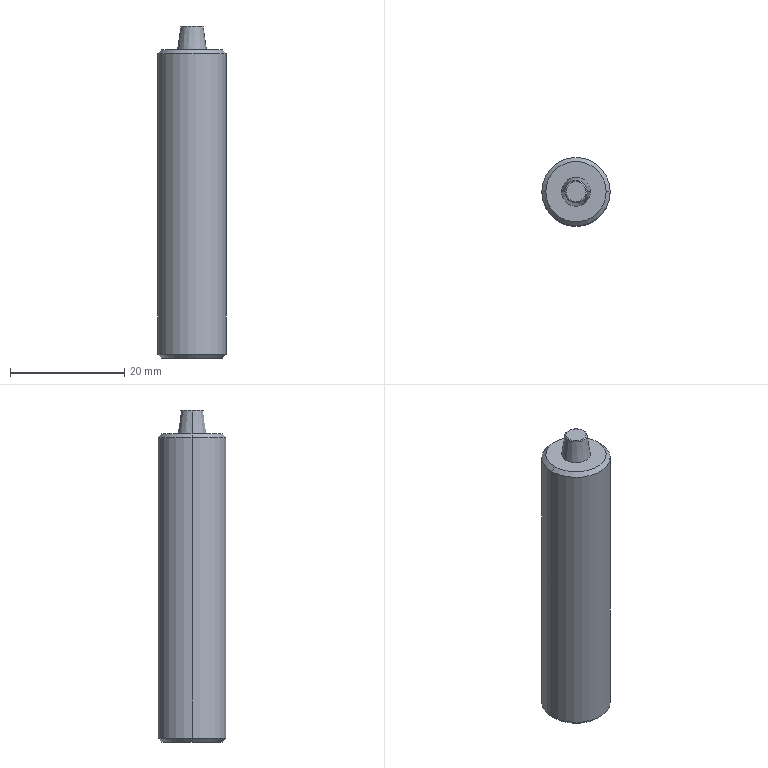Part | SolidWorks | features RefAxis 21, 3DProfileFeature 7, Revolution 3, ICE 2, RevCut 2 | 1 solid | 39 faces | box 12 x 12 x 58.2 mm | volume 5676 mm3 | plane 23 | cone 10 | cylinder 4 | torus 2 | commonest cylinder face diameters 6.917 x2 12 x2
STEP:
#1=CARTESIAN_POINT('',(0.,0.,-40.845));
#2=VERTEX_POINT('',#1);
#3=CARTESIAN_POINT('',(-2.,0.,-42.));
#4=VERTEX_POINT('',#3);
#5=CARTESIAN_POINT('',(-2.,0.,-42.));
#6=DIRECTION('',(-0.866,0.,-0.5));
#7=VECTOR('',#6,1000.);
#8=LINE('',#5,#7);
#9=EDGE_CURVE('',#2,#4,#8,.T.);
#10=ORIENTED_EDGE('',*,*,#9,.F.);
#11=CARTESIAN_POINT('',(2.,0.,-42.));
#12=VERTEX_POINT('',#11);
#13=CARTESIAN_POINT('',(2.,0.,-42.));
#14=DIRECTION('',(0.866,0.,-0.5));
#15=VECTOR('',#14,1000.);
#16=LINE('',#13,#15);
#17=EDGE_CURVE('',#2,#12,#16,.T.);
#18=ORIENTED_EDGE('',*,*,#17,.T.);
#19=CARTESIAN_POINT('',(1.,-1.732,-42.));
#20=VERTEX_POINT('',#19);
#21=CARTESIAN_POINT('',(0.,0.,-42.));
#22=DIRECTION('',(0.,0.,-1.));
#23=DIRECTION('',(1.,0.,0.));
#24=AXIS2_PLACEMENT_3D('',#21,#22,#23);
#25=CIRCLE('',#24,2.);
#26=EDGE_CURVE('',#12,#20,#25,.T.);
#27=ORIENTED_EDGE('',*,*,#26,.T.);
#28=CARTESIAN_POINT('',(-1.,-1.732,-42.));
#29=VERTEX_POINT('',#28);
#30=CARTESIAN_POINT('',(0.,0.,-42.));
#31=DIRECTION('',(0.,0.,-1.));
#32=DIRECTION('',(1.,0.,0.));
#33=AXIS2_PLACEMENT_3D('',#30,#31,#32);
#34=CIRCLE('',#33,2.);
#35=EDGE_CURVE('',#20,#29,#34,.T.);
#36=ORIENTED_EDGE('',*,*,#35,.T.);
#37=CARTESIAN_POINT('',(0.,0.,-42.));
#38=DIRECTION('',(0.,0.,-1.));
#39=DIRECTION('',(1.,0.,0.));
#40=AXIS2_PLACEMENT_3D('',#37,#38,#39);
#41=CIRCLE('',#40,2.);
#42=EDGE_CURVE('',#29,#4,#41,.T.);
#43=ORIENTED_EDGE('',*,*,#42,.T.);
#44=EDGE_LOOP('',(#10,#18,#27,#36,#43));
#45=FACE_OUTER_BOUND('',#44,.T.);
#46=CARTESIAN_POINT('',(0.,0.,-42.));
#47=DIRECTION('',(0.,0.,-1.));
#48=DIRECTION('',(-1.,0.,0.));
#49=AXIS2_PLACEMENT_3D('',#46,#47,#48);
#50=CONICAL_SURFACE('',#49,2.,1.047);
#51=ADVANCED_FACE('',(#45),#50,.F.);
#52=CARTESIAN_POINT('',(1.961,0.,4.028));
#53=VERTEX_POINT('',#52);
#54=CARTESIAN_POINT('',(-1.961,0.,4.028));
#55=VERTEX_POINT('',#54);
#56=CARTESIAN_POINT('',(0.,0.,4.028));
#57=DIRECTION('',(0.,0.,1.));
#58=DIRECTION('',(1.,0.,0.));
#59=AXIS2_PLACEMENT_3D('',#56,#57,#58);
#60=CIRCLE('',#59,1.961);
#61=EDGE_CURVE('',#53,#55,#60,.T.);
#62=ORIENTED_EDGE('',*,*,#61,.T.);
#63=CARTESIAN_POINT('',(-1.763,0.,4.2));
#64=VERTEX_POINT('',#63);
#65=CARTESIAN_POINT('',(-1.763,0.,4.));
#66=DIRECTION('',(0.,1.,0.));
#67=DIRECTION('',(-1.,0.,0.));
#68=AXIS2_PLACEMENT_3D('',#65,#66,#67);
#69=CIRCLE('',#68,0.2);
#70=EDGE_CURVE('',#55,#64,#69,.T.);
#71=ORIENTED_EDGE('',*,*,#70,.T.);
#72=CARTESIAN_POINT('',(1.763,0.,4.2));
#73=VERTEX_POINT('',#72);
#74=CARTESIAN_POINT('',(0.,0.,4.2));
#75=DIRECTION('',(0.,0.,1.));
#76=DIRECTION('',(1.,0.,0.));
#77=AXIS2_PLACEMENT_3D('',#74,#75,#76);
#78=CIRCLE('',#77,1.763);
#79=EDGE_CURVE('',#73,#64,#78,.T.);
#80=ORIENTED_EDGE('',*,*,#79,.F.);
#81=CARTESIAN_POINT('',(1.763,0.,4.));
#82=DIRECTION('',(0.,-1.,0.));
#83=DIRECTION('',(0.,0.,-1.));
#84=AXIS2_PLACEMENT_3D('',#81,#82,#83);
#85=CIRCLE('',#84,0.2);
#86=EDGE_CURVE('',#53,#73,#85,.T.);
#87=ORIENTED_EDGE('',*,*,#86,.F.);
#88=EDGE_LOOP('',(#62,#71,#80,#87));
#89=FACE_OUTER_BOUND('',#88,.T.);
#90=CARTESIAN_POINT('',(0.,0.,4.));
#91=DIRECTION('',(0.,0.,1.));
#92=DIRECTION('',(1.,0.,0.));
#93=AXIS2_PLACEMENT_3D('',#90,#91,#92);
#94=TOROIDAL_SURFACE('',#93,1.763,0.2);
#95=ADVANCED_FACE('',(#89),#94,.T.);
#96=ORIENTED_EDGE('',*,*,#61,.F.);
#97=CARTESIAN_POINT('',(2.527,0.,0.));
#98=VERTEX_POINT('',#97);
#99=CARTESIAN_POINT('',(2.85,0.,-2.3));
#100=DIRECTION('',(0.1392,0.,-0.9903));
#101=VECTOR('',#100,1000.);
#102=LINE('',#99,#101);
#103=EDGE_CURVE('',#53,#98,#102,.T.);
#104=ORIENTED_EDGE('',*,*,#103,.T.);
#105=CARTESIAN_POINT('',(-2.527,0.,0.));
#106=VERTEX_POINT('',#105);
#107=CARTESIAN_POINT('',(0.,0.,0.));
#108=DIRECTION('',(0.,0.,1.));
#109=DIRECTION('',(-1.,0.,0.));
#110=AXIS2_PLACEMENT_3D('',#107,#108,#109);
#111=CIRCLE('',#110,2.527);
#112=EDGE_CURVE('',#98,#106,#111,.T.);
#113=ORIENTED_EDGE('',*,*,#112,.T.);
#114=CARTESIAN_POINT('',(-2.85,0.,-2.3));
#115=DIRECTION('',(-0.1392,0.,-0.9903));
#116=VECTOR('',#115,1000.);
#117=LINE('',#114,#116);
#118=EDGE_CURVE('',#55,#106,#117,.T.);
#119=ORIENTED_EDGE('',*,*,#118,.F.);
#120=EDGE_LOOP('',(#96,#104,#113,#119));
#121=FACE_OUTER_BOUND('',#120,.T.);
#122=CARTESIAN_POINT('',(0.,0.,-2.3));
#123=DIRECTION('',(0.,0.,-1.));
#124=DIRECTION('',(-1.,0.,0.));
#125=AXIS2_PLACEMENT_3D('',#122,#123,#124);
#126=CONICAL_SURFACE('',#125,2.85,0.1396);
#127=ADVANCED_FACE('',(#121),#126,.T.);
#128=CARTESIAN_POINT('',(5.3,0.,-54.));
#129=VERTEX_POINT('',#128);
#130=CARTESIAN_POINT('',(-5.3,0.,-54.));
#131=VERTEX_POINT('',#130);
#132=CARTESIAN_POINT('',(0.,0.,-54.));
#133=DIRECTION('',(0.,0.,1.));
#134=DIRECTION('',(1.,0.,0.));
#135=AXIS2_PLACEMENT_3D('',#132,#133,#134);
#136=CIRCLE('',#135,5.3);
#137=EDGE_CURVE('',#129,#131,#136,.T.);
#138=ORIENTED_EDGE('',*,*,#137,.T.);
#139=CARTESIAN_POINT('',(-6.,0.,-53.3));
#140=VERTEX_POINT('',#139);
#141=CARTESIAN_POINT('',(-5.3,0.,-54.));
#142=DIRECTION('',(-0.7071,0.,0.7071));
#143=VECTOR('',#142,1000.);
#144=LINE('',#141,#143);
#145=EDGE_CURVE('',#131,#140,#144,.T.);
#146=ORIENTED_EDGE('',*,*,#145,.T.);
#147=CARTESIAN_POINT('',(6.,0.,-53.3));
#148=VERTEX_POINT('',#147);
#149=CARTESIAN_POINT('',(0.,0.,-53.3));
#150=DIRECTION('',(0.,0.,1.));
#151=DIRECTION('',(1.,0.,0.));
#152=AXIS2_PLACEMENT_3D('',#149,#150,#151);
#153=CIRCLE('',#152,6.);
#154=EDGE_CURVE('',#148,#140,#153,.T.);
#155=ORIENTED_EDGE('',*,*,#154,.F.);
#156=CARTESIAN_POINT('',(5.3,0.,-54.));
#157=DIRECTION('',(0.7071,0.,0.7071));
#158=VECTOR('',#157,1000.);
#159=LINE('',#156,#158);
#160=EDGE_CURVE('',#129,#148,#159,.T.);
#161=ORIENTED_EDGE('',*,*,#160,.F.);
#162=EDGE_LOOP('',(#138,#146,#155,#161));
#163=FACE_OUTER_BOUND('',#162,.T.);
#164=CARTESIAN_POINT('',(0.,0.,-54.));
#165=DIRECTION('',(0.,0.,1.));
#166=DIRECTION('',(1.,0.,0.));
#167=AXIS2_PLACEMENT_3D('',#164,#165,#166);
#168=CONICAL_SURFACE('',#167,5.3,0.7854);
#169=ADVANCED_FACE('',(#163),#168,.T.);
#170=ORIENTED_EDGE('',*,*,#154,.T.);
#171=CARTESIAN_POINT('',(-6.,0.,-0.7));
#172=VERTEX_POINT('',#171);
#173=CARTESIAN_POINT('',(-6.,0.,-54.));
#174=DIRECTION('',(0.,0.,1.));
#175=VECTOR('',#174,1000.);
#176=LINE('',#173,#175);
#177=EDGE_CURVE('',#140,#172,#176,.T.);
#178=ORIENTED_EDGE('',*,*,#177,.T.);
#179=CARTESIAN_POINT('',(6.,0.,-0.7));
#180=VERTEX_POINT('',#179);
#181=CARTESIAN_POINT('',(0.,0.,-0.7));
#182=DIRECTION('',(0.,0.,1.));
#183=DIRECTION('',(1.,0.,0.));
#184=AXIS2_PLACEMENT_3D('',#181,#182,#183);
#185=CIRCLE('',#184,6.);
#186=EDGE_CURVE('',#180,#172,#185,.T.);
#187=ORIENTED_EDGE('',*,*,#186,.F.);
#188=CARTESIAN_POINT('',(6.,0.,-54.));
#189=DIRECTION('',(0.,0.,1.));
#190=VECTOR('',#189,1000.);
#191=LINE('',#188,#190);
#192=EDGE_CURVE('',#148,#180,#191,.T.);
#193=ORIENTED_EDGE('',*,*,#192,.F.);
#194=EDGE_LOOP('',(#170,#178,#187,#193));
#195=FACE_OUTER_BOUND('',#194,.T.);
#196=CARTESIAN_POINT('',(0.,0.,-54.));
#197=DIRECTION('',(0.,0.,1.));
#198=DIRECTION('',(1.,0.,0.));
#199=AXIS2_PLACEMENT_3D('',#196,#197,#198);
#200=CYLINDRICAL_SURFACE('',#199,6.);
#201=ADVANCED_FACE('',(#195),#200,.T.);
#202=CARTESIAN_POINT('',(5.3,0.,0.));
#203=VERTEX_POINT('',#202);
#204=CARTESIAN_POINT('',(-5.3,0.,0.));
#205=VERTEX_POINT('',#204);
#206=CARTESIAN_POINT('',(0.,0.,0.));
#207=DIRECTION('',(0.,0.,1.));
#208=DIRECTION('',(1.,0.,0.));
#209=AXIS2_PLACEMENT_3D('',#206,#207,#208);
#210=CIRCLE('',#209,5.3);
#211=EDGE_CURVE('',#203,#205,#210,.T.);
#212=ORIENTED_EDGE('',*,*,#211,.F.);
#213=CARTESIAN_POINT('',(6.,0.,-0.7));
#214=DIRECTION('',(0.7071,0.,-0.7071));
#215=VECTOR('',#214,1000.);
#216=LINE('',#213,#215);
#217=EDGE_CURVE('',#203,#180,#216,.T.);
#218=ORIENTED_EDGE('',*,*,#217,.T.);
#219=ORIENTED_EDGE('',*,*,#186,.T.);
#220=CARTESIAN_POINT('',(-6.,0.,-0.7));
#221=DIRECTION('',(-0.7071,0.,-0.7071));
#222=VECTOR('',#221,1000.);
#223=LINE('',#220,#222);
#224=EDGE_CURVE('',#205,#172,#223,.T.);
#225=ORIENTED_EDGE('',*,*,#224,.F.);
#226=EDGE_LOOP('',(#212,#218,#219,#225));
#227=FACE_OUTER_BOUND('',#226,.T.);
#228=CARTESIAN_POINT('',(0.,0.,-0.7));
#229=DIRECTION('',(0.,0.,-1.));
#230=DIRECTION('',(-1.,0.,0.));
#231=AXIS2_PLACEMENT_3D('',#228,#229,#230);
#232=CONICAL_SURFACE('',#231,6.,0.7854);
#233=ADVANCED_FACE('',(#227),#232,.T.);
#234=CARTESIAN_POINT('',(4.,-2.309,-53.819));
#235=VERTEX_POINT('',#234);
#236=CARTESIAN_POINT('',(4.,0.,-53.2));
#237=VERTEX_POINT('',#236);
#238=CARTESIAN_POINT('',(4.,-2.309,-53.819));
#239=CARTESIAN_POINT('',(4.,-1.951,-53.64));
#240=CARTESIAN_POINT('',(4.,-1.574,-53.483));
#241=CARTESIAN_POINT('',(4.,-0.9966,-53.318));
#242=CARTESIAN_POINT('',(4.,-0.8015,-53.275));
#243=CARTESIAN_POINT('',(4.,-0.4053,-53.216));
#244=CARTESIAN_POINT('',(4.,-0.2027,-53.2));
#245=CARTESIAN_POINT('',(4.,0.,-53.2));
#246=B_SPLINE_CURVE_WITH_KNOTS('',3,(#238,#239,#240,#241,#242,#243,#244,#245),.UNSPECIFIED.,.F.,.F.,(4,2,2,4),(0.003092,0.004289,0.004887,0.005485),.UNSPECIFIED.);
#247=EDGE_CURVE('',#235,#237,#246,.T.);
#248=ORIENTED_EDGE('',*,*,#247,.T.);
#249=CARTESIAN_POINT('',(4.8,0.,-54.));
#250=VERTEX_POINT('',#249);
#251=CARTESIAN_POINT('',(4.8,0.,-54.));
#252=DIRECTION('',(0.7071,0.,-0.7071));
#253=VECTOR('',#252,1000.);
#254=LINE('',#251,#253);
#255=EDGE_CURVE('',#237,#250,#254,.T.);
#256=ORIENTED_EDGE('',*,*,#255,.T.);
#257=CARTESIAN_POINT('',(-4.8,0.,-54.));
#258=VERTEX_POINT('',#257);
#259=CARTESIAN_POINT('',(0.,0.,-54.));
#260=DIRECTION('',(0.,0.,1.));
#261=DIRECTION('',(1.,0.,0.));
#262=AXIS2_PLACEMENT_3D('',#259,#260,#261);
#263=CIRCLE('',#262,4.8);
#264=EDGE_CURVE('',#258,#250,#263,.T.);
#265=ORIENTED_EDGE('',*,*,#264,.F.);
#266=CARTESIAN_POINT('',(-4.,0.,-53.2));
#267=VERTEX_POINT('',#266);
#268=CARTESIAN_POINT('',(-4.8,0.,-54.));
#269=DIRECTION('',(-0.7071,0.,-0.7071));
#270=VECTOR('',#269,1000.);
#271=LINE('',#268,#270);
#272=EDGE_CURVE('',#267,#258,#271,.T.);
#273=ORIENTED_EDGE('',*,*,#272,.F.);
#274=CARTESIAN_POINT('',(-4.,-2.309,-53.819));
#275=VERTEX_POINT('',#274);
#276=CARTESIAN_POINT('',(-4.,0.,-53.2));
#277=CARTESIAN_POINT('',(-4.,-0.2027,-53.2));
#278=CARTESIAN_POINT('',(-4.,-0.4053,-53.216));
#279=CARTESIAN_POINT('',(-4.,-0.8015,-53.275));
#280=CARTESIAN_POINT('',(-4.,-0.9966,-53.318));
#281=CARTESIAN_POINT('',(-4.,-1.574,-53.483));
#282=CARTESIAN_POINT('',(-4.,-1.951,-53.64));
#283=CARTESIAN_POINT('',(-4.,-2.309,-53.819));
#284=B_SPLINE_CURVE_WITH_KNOTS('',3,(#276,#277,#278,#279,#280,#281,#282,#283),.UNSPECIFIED.,.F.,.F.,(4,2,2,4),(0.004837,0.005435,0.006033,0.007228),.UNSPECIFIED.);
#285=EDGE_CURVE('',#267,#275,#284,.T.);
#286=ORIENTED_EDGE('',*,*,#285,.T.);
#287=CARTESIAN_POINT('',(0.,-4.619,-53.819));
#288=VERTEX_POINT('',#287);
#289=CARTESIAN_POINT('',(-4.,-2.309,-53.819));
#290=CARTESIAN_POINT('',(-3.687,-2.49,-53.638));
#291=CARTESIAN_POINT('',(-3.368,-2.674,-53.485));
#292=CARTESIAN_POINT('',(-2.871,-2.961,-53.321));
#293=CARTESIAN_POINT('',(-2.703,-3.058,-53.277));
#294=CARTESIAN_POINT('',(-2.359,-3.257,-53.217));
#295=CARTESIAN_POINT('',(-2.182,-3.359,-53.2));
#296=CARTESIAN_POINT('',(-1.658,-3.661,-53.199));
#297=CARTESIAN_POINT('',(-1.315,-3.86,-53.26));
#298=CARTESIAN_POINT('',(-0.6381,-4.25,-53.482));
#299=CARTESIAN_POINT('',(-0.3144,-4.437,-53.637));
#300=CARTESIAN_POINT('',(0.,-4.619,-53.819));
#301=B_SPLINE_CURVE_WITH_KNOTS('',3,(#289,#290,#291,#292,#293,#294,#295,#296,#297,#298,#299,#300),.UNSPECIFIED.,.F.,.F.,(4,2,2,2,2,4),(0.000000254,0.001193,0.001789,0.002386,0.003579,0.004771),.UNSPECIFIED.);
#302=EDGE_CURVE('',#275,#288,#301,.T.);
#303=ORIENTED_EDGE('',*,*,#302,.T.);
#304=CARTESIAN_POINT('',(0.,-4.619,-53.819));
#305=CARTESIAN_POINT('',(0.3125,-4.438,-53.638));
#306=CARTESIAN_POINT('',(0.6321,-4.254,-53.485));
#307=CARTESIAN_POINT('',(1.129,-3.967,-53.321));
#308=CARTESIAN_POINT('',(1.297,-3.87,-53.277));
#309=CARTESIAN_POINT('',(1.641,-3.671,-53.217));
#310=CARTESIAN_POINT('',(1.818,-3.569,-53.2));
#311=CARTESIAN_POINT('',(2.342,-3.267,-53.199));
#312=CARTESIAN_POINT('',(2.685,-3.069,-53.26));
#313=CARTESIAN_POINT('',(3.362,-2.678,-53.482));
#314=CARTESIAN_POINT('',(3.686,-2.491,-53.637));
#315=CARTESIAN_POINT('',(4.,-2.309,-53.819));
#316=B_SPLINE_CURVE_WITH_KNOTS('',3,(#304,#305,#306,#307,#308,#309,#310,#311,#312,#313,#314,#315),.UNSPECIFIED.,.F.,.F.,(4,2,2,2,2,4),(0.000000254,0.001193,0.001789,0.002386,0.003579,0.004771),.UNSPECIFIED.);
#317=EDGE_CURVE('',#288,#235,#316,.T.);
#318=ORIENTED_EDGE('',*,*,#317,.T.);
#319=EDGE_LOOP('',(#248,#256,#265,#273,#286,#303,#318));
#320=FACE_OUTER_BOUND('',#319,.T.);
#321=CARTESIAN_POINT('',(0.,0.,-54.));
#322=DIRECTION('',(0.,0.,-1.));
#323=DIRECTION('',(-1.,0.,0.));
#324=AXIS2_PLACEMENT_3D('',#321,#322,#323);
#325=CONICAL_SURFACE('',#324,4.8,0.7854);
#326=ADVANCED_FACE('',(#320),#325,.F.);
#327=CARTESIAN_POINT('',(-3.458,0.,-49.));
#328=VERTEX_POINT('',#327);
#329=CARTESIAN_POINT('',(3.458,0.,-49.));
#330=VERTEX_POINT('',#329);
#331=CARTESIAN_POINT('',(0.,0.,-49.));
#332=DIRECTION('',(0.,0.,1.));
#333=DIRECTION('',(1.,0.,0.));
#334=AXIS2_PLACEMENT_3D('',#331,#332,#333);
#335=CIRCLE('',#334,3.458);
#336=EDGE_CURVE('',#328,#330,#335,.T.);
#337=ORIENTED_EDGE('',*,*,#336,.F.);
#338=CARTESIAN_POINT('',(-3.458,0.,-45.));
#339=VERTEX_POINT('',#338);
#340=CARTESIAN_POINT('',(-3.458,0.,-54.));
#341=DIRECTION('',(0.,0.,1.));
#342=VECTOR('',#341,1000.);
#343=LINE('',#340,#342);
#344=EDGE_CURVE('',#328,#339,#343,.T.);
#345=ORIENTED_EDGE('',*,*,#344,.T.);
#346=CARTESIAN_POINT('',(3.458,0.,-45.));
#347=VERTEX_POINT('',#346);
#348=CARTESIAN_POINT('',(0.,0.,-45.));
#349=DIRECTION('',(0.,0.,1.));
#350=DIRECTION('',(1.,0.,0.));
#351=AXIS2_PLACEMENT_3D('',#348,#349,#350);
#352=CIRCLE('',#351,3.458);
#353=EDGE_CURVE('',#339,#347,#352,.T.);
#354=ORIENTED_EDGE('',*,*,#353,.T.);
#355=CARTESIAN_POINT('',(3.458,0.,-54.));
#356=DIRECTION('',(0.,0.,1.));
#357=VECTOR('',#356,1000.);
#358=LINE('',#355,#357);
#359=EDGE_CURVE('',#330,#347,#358,.T.);
#360=ORIENTED_EDGE('',*,*,#359,.F.);
#361=EDGE_LOOP('',(#337,#345,#354,#360));
#362=FACE_OUTER_BOUND('',#361,.T.);
#363=CARTESIAN_POINT('',(0.,0.,-54.));
#364=DIRECTION('',(0.,0.,1.));
#365=DIRECTION('',(1.,0.,0.));
#366=AXIS2_PLACEMENT_3D('',#363,#364,#365);
#367=CYLINDRICAL_SURFACE('',#366,3.458);
#368=ADVANCED_FACE('',(#362),#367,.F.);
#369=ORIENTED_EDGE('',*,*,#26,.F.);
#370=CARTESIAN_POINT('',(2.,-1.155,-42.));
#371=VERTEX_POINT('',#370);
#372=CARTESIAN_POINT('',(2.,-1.155,-42.));
#373=DIRECTION('',(0.,1.,0.));
#374=VECTOR('',#373,1000.);
#375=LINE('',#372,#374);
#376=EDGE_CURVE('',#371,#12,#375,.T.);
#377=ORIENTED_EDGE('',*,*,#376,.F.);
#378=CARTESIAN_POINT('',(0.,-2.309,-42.));
#379=DIRECTION('',(0.866,0.5,0.));
#380=VECTOR('',#379,1000.);
#381=LINE('',#378,#380);
#382=EDGE_CURVE('',#20,#371,#381,.T.);
#383=ORIENTED_EDGE('',*,*,#382,.F.);
#384=EDGE_LOOP('',(#369,#377,#383));
#385=FACE_OUTER_BOUND('',#384,.T.);
#386=CARTESIAN_POINT('',(0.,0.,-42.));
#387=DIRECTION('',(0.,0.,1.));
#388=DIRECTION('',(1.,0.,0.));
#389=AXIS2_PLACEMENT_3D('',#386,#387,#388);
#390=PLANE('',#389);
#391=ADVANCED_FACE('',(#385),#390,.F.);
#392=ORIENTED_EDGE('',*,*,#35,.F.);
#393=CARTESIAN_POINT('',(0.,-2.309,-42.));
#394=VERTEX_POINT('',#393);
#395=CARTESIAN_POINT('',(0.,-2.309,-42.));
#396=DIRECTION('',(0.866,0.5,0.));
#397=VECTOR('',#396,1000.);
#398=LINE('',#395,#397);
#399=EDGE_CURVE('',#394,#20,#398,.T.);
#400=ORIENTED_EDGE('',*,*,#399,.F.);
#401=CARTESIAN_POINT('',(-2.,-1.155,-42.));
#402=DIRECTION('',(0.866,-0.5,0.));
#403=VECTOR('',#402,1000.);
#404=LINE('',#401,#403);
#405=EDGE_CURVE('',#29,#394,#404,.T.);
#406=ORIENTED_EDGE('',*,*,#405,.F.);
#407=EDGE_LOOP('',(#392,#400,#406));
#408=FACE_OUTER_BOUND('',#407,.T.);
#409=CARTESIAN_POINT('',(0.,0.,-42.));
#410=DIRECTION('',(0.,0.,1.));
#411=DIRECTION('',(1.,0.,0.));
#412=AXIS2_PLACEMENT_3D('',#409,#410,#411);
#413=PLANE('',#412);
#414=ADVANCED_FACE('',(#408),#413,.F.);
#415=ORIENTED_EDGE('',*,*,#42,.F.);
#416=CARTESIAN_POINT('',(-2.,-1.155,-42.));
#417=VERTEX_POINT('',#416);
#418=CARTESIAN_POINT('',(-2.,-1.155,-42.));
#419=DIRECTION('',(0.866,-0.5,0.));
#420=VECTOR('',#419,1000.);
#421=LINE('',#418,#420);
#422=EDGE_CURVE('',#417,#29,#421,.T.);
#423=ORIENTED_EDGE('',*,*,#422,.F.);
#424=CARTESIAN_POINT('',(-2.,1.155,-42.));
#425=DIRECTION('',(0.,-1.,0.));
#426=VECTOR('',#425,1000.);
#427=LINE('',#424,#426);
#428=EDGE_CURVE('',#4,#417,#427,.T.);
#429=ORIENTED_EDGE('',*,*,#428,.F.);
#430=EDGE_LOOP('',(#415,#423,#429));
#431=FACE_OUTER_BOUND('',#430,.T.);
#432=CARTESIAN_POINT('',(0.,0.,-42.));
#433=DIRECTION('',(0.,0.,1.));
#434=DIRECTION('',(1.,0.,0.));
#435=AXIS2_PLACEMENT_3D('',#432,#433,#434);
#436=PLANE('',#435);
#437=ADVANCED_FACE('',(#431),#436,.F.);
#438=CARTESIAN_POINT('',(-1.,1.732,-42.));
#439=VERTEX_POINT('',#438);
#440=CARTESIAN_POINT('',(0.,0.,-42.));
#441=DIRECTION('',(0.,0.,-1.));
#442=DIRECTION('',(1.,0.,0.));
#443=AXIS2_PLACEMENT_3D('',#440,#441,#442);
#444=CIRCLE('',#443,2.);
#445=EDGE_CURVE('',#4,#439,#444,.T.);
#446=ORIENTED_EDGE('',*,*,#445,.F.);
#447=CARTESIAN_POINT('',(-2.,1.155,-42.));
#448=VERTEX_POINT('',#447);
#449=CARTESIAN_POINT('',(-2.,1.155,-42.));
#450=DIRECTION('',(0.,-1.,0.));
#451=VECTOR('',#450,1000.);
#452=LINE('',#449,#451);
#453=EDGE_CURVE('',#448,#4,#452,.T.);
#454=ORIENTED_EDGE('',*,*,#453,.F.);
#455=CARTESIAN_POINT('',(0.,2.309,-42.));
#456=DIRECTION('',(-0.866,-0.5,0.));
#457=VECTOR('',#456,1000.);
#458=LINE('',#455,#457);
#459=EDGE_CURVE('',#439,#448,#458,.T.);
#460=ORIENTED_EDGE('',*,*,#459,.F.);
#461=EDGE_LOOP('',(#446,#454,#460));
#462=FACE_OUTER_BOUND('',#461,.T.);
#463=CARTESIAN_POINT('',(0.,0.,-42.));
#464=DIRECTION('',(0.,0.,1.));
#465=DIRECTION('',(1.,0.,0.));
#466=AXIS2_PLACEMENT_3D('',#463,#464,#465);
#467=PLANE('',#466);
#468=ADVANCED_FACE('',(#462),#467,.F.);
#469=CARTESIAN_POINT('',(1.,1.732,-42.));
#470=VERTEX_POINT('',#469);
#471=CARTESIAN_POINT('',(0.,0.,-42.));
#472=DIRECTION('',(0.,0.,-1.));
#473=DIRECTION('',(1.,0.,0.));
#474=AXIS2_PLACEMENT_3D('',#471,#472,#473);
#475=CIRCLE('',#474,2.);
#476=EDGE_CURVE('',#439,#470,#475,.T.);
#477=ORIENTED_EDGE('',*,*,#476,.F.);
#478=CARTESIAN_POINT('',(0.,2.309,-42.));
#479=VERTEX_POINT('',#478);
#480=CARTESIAN_POINT('',(0.,2.309,-42.));
#481=DIRECTION('',(-0.866,-0.5,0.));
#482=VECTOR('',#481,1000.);
#483=LINE('',#480,#482);
#484=EDGE_CURVE('',#479,#439,#483,.T.);
#485=ORIENTED_EDGE('',*,*,#484,.F.);
#486=CARTESIAN_POINT('',(2.,1.155,-42.));
#487=DIRECTION('',(-0.866,0.5,0.));
#488=VECTOR('',#487,1000.);
#489=LINE('',#486,#488);
#490=EDGE_CURVE('',#470,#479,#489,.T.);
#491=ORIENTED_EDGE('',*,*,#490,.F.);
#492=EDGE_LOOP('',(#477,#485,#491));
#493=FACE_OUTER_BOUND('',#492,.T.);
#494=CARTESIAN_POINT('',(0.,0.,-42.));
#495=DIRECTION('',(0.,0.,1.));
#496=DIRECTION('',(1.,0.,0.));
#497=AXIS2_PLACEMENT_3D('',#494,#495,#496);
#498=PLANE('',#497);
#499=ADVANCED_FACE('',(#493),#498,.F.);
#500=CARTESIAN_POINT('',(0.,0.,-42.));
#501=DIRECTION('',(0.,0.,1.));
#502=DIRECTION('',(1.,0.,0.));
#503=AXIS2_PLACEMENT_3D('',#500,#501,#502);
#504=CIRCLE('',#503,2.);
#505=EDGE_CURVE('',#12,#470,#504,.T.);
#506=ORIENTED_EDGE('',*,*,#505,.T.);
#507=CARTESIAN_POINT('',(2.,1.155,-42.));
#508=VERTEX_POINT('',#507);
#509=CARTESIAN_POINT('',(2.,1.155,-42.));
#510=DIRECTION('',(-0.866,0.5,0.));
#511=VECTOR('',#510,1000.);
#512=LINE('',#509,#511);
#513=EDGE_CURVE('',#508,#470,#512,.T.);
#514=ORIENTED_EDGE('',*,*,#513,.F.);
#515=CARTESIAN_POINT('',(2.,-1.155,-42.));
#516=DIRECTION('',(0.,1.,0.));
#517=VECTOR('',#516,1000.);
#518=LINE('',#515,#517);
#519=EDGE_CURVE('',#12,#508,#518,.T.);
#520=ORIENTED_EDGE('',*,*,#519,.F.);
#521=EDGE_LOOP('',(#506,#514,#520));
#522=FACE_OUTER_BOUND('',#521,.T.);
#523=CARTESIAN_POINT('',(0.,0.,-42.));
#524=DIRECTION('',(0.,0.,1.));
#525=DIRECTION('',(1.,0.,0.));
#526=AXIS2_PLACEMENT_3D('',#523,#524,#525);
#527=PLANE('',#526);
#528=ADVANCED_FACE('',(#522),#527,.F.);
#529=CARTESIAN_POINT('',(0.,0.,-45.));
#530=DIRECTION('',(0.,0.,1.));
#531=DIRECTION('',(1.,0.,0.));
#532=AXIS2_PLACEMENT_3D('',#529,#530,#531);
#533=CIRCLE('',#532,3.458);
#534=EDGE_CURVE('',#347,#339,#533,.T.);
#535=ORIENTED_EDGE('',*,*,#534,.F.);
#536=ORIENTED_EDGE('',*,*,#353,.F.);
#537=EDGE_LOOP('',(#535,#536));
#538=FACE_OUTER_BOUND('',#537,.T.);
#539=CARTESIAN_POINT('',(-2.,1.155,-45.));
#540=VERTEX_POINT('',#539);
#541=CARTESIAN_POINT('',(-2.,-1.155,-45.));
#542=VERTEX_POINT('',#541);
#543=CARTESIAN_POINT('',(-2.,1.155,-45.));
#544=DIRECTION('',(0.,-1.,0.));
#545=VECTOR('',#544,1000.);
#546=LINE('',#543,#545);
#547=EDGE_CURVE('',#540,#542,#546,.T.);
#548=ORIENTED_EDGE('',*,*,#547,.T.);
#549=CARTESIAN_POINT('',(0.,-2.309,-45.));
#550=VERTEX_POINT('',#549);
#551=CARTESIAN_POINT('',(-2.,-1.155,-45.));
#552=DIRECTION('',(0.866,-0.5,0.));
#553=VECTOR('',#552,1000.);
#554=LINE('',#551,#553);
#555=EDGE_CURVE('',#542,#550,#554,.T.);
#556=ORIENTED_EDGE('',*,*,#555,.T.);
#557=CARTESIAN_POINT('',(2.,-1.155,-45.));
#558=VERTEX_POINT('',#557);
#559=CARTESIAN_POINT('',(0.,-2.309,-45.));
#560=DIRECTION('',(0.866,0.5,0.));
#561=VECTOR('',#560,1000.);
#562=LINE('',#559,#561);
#563=EDGE_CURVE('',#550,#558,#562,.T.);
#564=ORIENTED_EDGE('',*,*,#563,.T.);
#565=CARTESIAN_POINT('',(2.,1.155,-45.));
#566=VERTEX_POINT('',#565);
#567=CARTESIAN_POINT('',(2.,-1.155,-45.));
#568=DIRECTION('',(0.,1.,0.));
#569=VECTOR('',#568,1000.);
#570=LINE('',#567,#569);
#571=EDGE_CURVE('',#558,#566,#570,.T.);
#572=ORIENTED_EDGE('',*,*,#571,.T.);
#573=CARTESIAN_POINT('',(0.,2.309,-45.));
#574=VERTEX_POINT('',#573);
#575=CARTESIAN_POINT('',(2.,1.155,-45.));
#576=DIRECTION('',(-0.866,0.5,0.));
#577=VECTOR('',#576,1000.);
#578=LINE('',#575,#577);
#579=EDGE_CURVE('',#566,#574,#578,.T.);
#580=ORIENTED_EDGE('',*,*,#579,.T.);
#581=CARTESIAN_POINT('',(0.,2.309,-45.));
#582=DIRECTION('',(-0.866,-0.5,0.));
#583=VECTOR('',#582,1000.);
#584=LINE('',#581,#583);
#585=EDGE_CURVE('',#574,#540,#584,.T.);
#586=ORIENTED_EDGE('',*,*,#585,.T.);
#587=EDGE_LOOP('',(#548,#556,#564,#572,#580,#586));
#588=FACE_BOUND('',#587,.T.);
#589=CARTESIAN_POINT('',(0.,4.,-45.));
#590=DIRECTION('',(0.,0.,1.));
#591=DIRECTION('',(1.,0.,0.));
#592=AXIS2_PLACEMENT_3D('',#589,#590,#591);
#593=PLANE('',#592);
#594=ADVANCED_FACE('',(#538,#588),#593,.F.);
#595=ORIENTED_EDGE('',*,*,#344,.F.);
#596=CARTESIAN_POINT('',(0.,0.,-49.));
#597=DIRECTION('',(0.,0.,1.));
#598=DIRECTION('',(1.,0.,0.));
#599=AXIS2_PLACEMENT_3D('',#596,#597,#598);
#600=CIRCLE('',#599,3.458);
#601=EDGE_CURVE('',#330,#328,#600,.T.);
#602=ORIENTED_EDGE('',*,*,#601,.F.);
#603=ORIENTED_EDGE('',*,*,#359,.T.);
#604=ORIENTED_EDGE('',*,*,#534,.T.);
#605=EDGE_LOOP('',(#595,#602,#603,#604));
#606=FACE_OUTER_BOUND('',#605,.T.);
#607=CARTESIAN_POINT('',(0.,0.,-54.));
#608=DIRECTION('',(0.,0.,1.));
#609=DIRECTION('',(1.,0.,0.));
#610=AXIS2_PLACEMENT_3D('',#607,#608,#609);
#611=CYLINDRICAL_SURFACE('',#610,3.458);
#612=ADVANCED_FACE('',(#606),#611,.F.);
#613=ORIENTED_EDGE('',*,*,#255,.F.);
#614=CARTESIAN_POINT('',(4.,2.309,-53.819));
#615=VERTEX_POINT('',#614);
#616=CARTESIAN_POINT('',(4.,0.,-53.2));
#617=CARTESIAN_POINT('',(4.,0.4059,-53.2));
#618=CARTESIAN_POINT('',(4.,0.8013,-53.263));
#619=CARTESIAN_POINT('',(4.,1.382,-53.428));
#620=CARTESIAN_POINT('',(4.,1.575,-53.495));
#621=CARTESIAN_POINT('',(4.,1.948,-53.646));
#622=CARTESIAN_POINT('',(4.,2.131,-53.729));
#623=CARTESIAN_POINT('',(4.,2.309,-53.819));
#624=B_SPLINE_CURVE_WITH_KNOTS('',3,(#616,#617,#618,#619,#620,#621,#622,#623),.UNSPECIFIED.,.F.,.F.,(4,2,2,4),(0.005485,0.006683,0.007282,0.007881),.UNSPECIFIED.);
#625=EDGE_CURVE('',#237,#615,#624,.T.);
#626=ORIENTED_EDGE('',*,*,#625,.T.);
#627=CARTESIAN_POINT('',(0.,4.619,-53.819));
#628=VERTEX_POINT('',#627);
#629=CARTESIAN_POINT('',(4.,2.309,-53.819));
#630=CARTESIAN_POINT('',(3.687,2.49,-53.638));
#631=CARTESIAN_POINT('',(3.368,2.674,-53.485));
#632=CARTESIAN_POINT('',(2.871,2.961,-53.321));
#633=CARTESIAN_POINT('',(2.703,3.058,-53.277));
#634=CARTESIAN_POINT('',(2.359,3.257,-53.217));
#635=CARTESIAN_POINT('',(2.182,3.359,-53.2));
#636=CARTESIAN_POINT('',(1.658,3.661,-53.199));
#637=CARTESIAN_POINT('',(1.315,3.86,-53.26));
#638=CARTESIAN_POINT('',(0.6381,4.25,-53.482));
#639=CARTESIAN_POINT('',(0.3144,4.437,-53.637));
#640=CARTESIAN_POINT('',(0.,4.619,-53.819));
#641=B_SPLINE_CURVE_WITH_KNOTS('',3,(#629,#630,#631,#632,#633,#634,#635,#636,#637,#638,#639,#640),.UNSPECIFIED.,.F.,.F.,(4,2,2,2,2,4),(0.000000254,0.001193,0.001789,0.002386,0.003579,0.004771),.UNSPECIFIED.);
#642=EDGE_CURVE('',#615,#628,#641,.T.);
#643=ORIENTED_EDGE('',*,*,#642,.T.);
#644=CARTESIAN_POINT('',(-4.,2.309,-53.819));
#645=VERTEX_POINT('',#644);
#646=CARTESIAN_POINT('',(0.,4.619,-53.819));
#647=CARTESIAN_POINT('',(-0.3125,4.438,-53.638));
#648=CARTESIAN_POINT('',(-0.6321,4.254,-53.485));
#649=CARTESIAN_POINT('',(-1.129,3.967,-53.321));
#650=CARTESIAN_POINT('',(-1.297,3.87,-53.277));
#651=CARTESIAN_POINT('',(-1.641,3.671,-53.217));
#652=CARTESIAN_POINT('',(-1.818,3.569,-53.2));
#653=CARTESIAN_POINT('',(-2.342,3.267,-53.199));
#654=CARTESIAN_POINT('',(-2.685,3.069,-53.26));
#655=CARTESIAN_POINT('',(-3.362,2.678,-53.482));
#656=CARTESIAN_POINT('',(-3.686,2.491,-53.637));
#657=CARTESIAN_POINT('',(-4.,2.309,-53.819));
#658=B_SPLINE_CURVE_WITH_KNOTS('',3,(#646,#647,#648,#649,#650,#651,#652,#653,#654,#655,#656,#657),.UNSPECIFIED.,.F.,.F.,(4,2,2,2,2,4),(0.000000254,0.001193,0.001789,0.002386,0.003579,0.004771),.UNSPECIFIED.);
#659=EDGE_CURVE('',#628,#645,#658,.T.);
#660=ORIENTED_EDGE('',*,*,#659,.T.);
#661=CARTESIAN_POINT('',(-4.,2.309,-53.819));
#662=CARTESIAN_POINT('',(-4.,2.131,-53.729));
#663=CARTESIAN_POINT('',(-4.,1.948,-53.646));
#664=CARTESIAN_POINT('',(-4.,1.575,-53.495));
#665=CARTESIAN_POINT('',(-4.,1.382,-53.428));
#666=CARTESIAN_POINT('',(-4.,0.8013,-53.263));
#667=CARTESIAN_POINT('',(-4.,0.4059,-53.2));
#668=CARTESIAN_POINT('',(-4.,0.,-53.2));
#669=B_SPLINE_CURVE_WITH_KNOTS('',3,(#661,#662,#663,#664,#665,#666,#667,#668),.UNSPECIFIED.,.F.,.F.,(4,2,2,4),(0.002443,0.003041,0.00364,0.004837),.UNSPECIFIED.);
#670=EDGE_CURVE('',#645,#267,#669,.T.);
#671=ORIENTED_EDGE('',*,*,#670,.T.);
#672=ORIENTED_EDGE('',*,*,#272,.T.);
#673=CARTESIAN_POINT('',(0.,0.,-54.));
#674=DIRECTION('',(0.,0.,1.));
#675=DIRECTION('',(1.,0.,0.));
#676=AXIS2_PLACEMENT_3D('',#673,#674,#675);
#677=CIRCLE('',#676,4.8);
#678=EDGE_CURVE('',#250,#258,#677,.T.);
#679=ORIENTED_EDGE('',*,*,#678,.F.);
#680=EDGE_LOOP('',(#613,#626,#643,#660,#671,#672,#679));
#681=FACE_OUTER_BOUND('',#680,.T.);
#682=CARTESIAN_POINT('',(0.,0.,-54.));
#683=DIRECTION('',(0.,0.,-1.));
#684=DIRECTION('',(-1.,0.,0.));
#685=AXIS2_PLACEMENT_3D('',#682,#683,#684);
#686=CONICAL_SURFACE('',#685,4.8,0.7854);
#687=ADVANCED_FACE('',(#681),#686,.F.);
#688=CARTESIAN_POINT('',(0.,0.,0.));
#689=DIRECTION('',(0.,0.,1.));
#690=DIRECTION('',(1.,0.,0.));
#691=AXIS2_PLACEMENT_3D('',#688,#689,#690);
#692=CIRCLE('',#691,5.3);
#693=EDGE_CURVE('',#205,#203,#692,.T.);
#694=ORIENTED_EDGE('',*,*,#693,.T.);
#695=ORIENTED_EDGE('',*,*,#211,.T.);
#696=EDGE_LOOP('',(#694,#695));
#697=FACE_OUTER_BOUND('',#696,.T.);
#698=CARTESIAN_POINT('',(0.,0.,0.));
#699=DIRECTION('',(0.,0.,1.));
#700=DIRECTION('',(-1.,0.,0.));
#701=AXIS2_PLACEMENT_3D('',#698,#699,#700);
#702=CIRCLE('',#701,2.527);
#703=EDGE_CURVE('',#106,#98,#702,.T.);
#704=ORIENTED_EDGE('',*,*,#703,.F.);
#705=ORIENTED_EDGE('',*,*,#112,.F.);
#706=EDGE_LOOP('',(#704,#705));
#707=FACE_BOUND('',#706,.T.);
#708=CARTESIAN_POINT('',(0.,0.,0.));
#709=DIRECTION('',(0.,0.,-1.));
#710=DIRECTION('',(-1.,0.,0.));
#711=AXIS2_PLACEMENT_3D('',#708,#709,#710);
#712=PLANE('',#711);
#713=ADVANCED_FACE('',(#697,#707),#712,.F.);
#714=ORIENTED_EDGE('',*,*,#137,.F.);
#715=CARTESIAN_POINT('',(0.,0.,-54.));
#716=DIRECTION('',(0.,0.,1.));
#717=DIRECTION('',(1.,0.,0.));
#718=AXIS2_PLACEMENT_3D('',#715,#716,#717);
#719=CIRCLE('',#718,5.3);
#720=EDGE_CURVE('',#131,#129,#719,.T.);
#721=ORIENTED_EDGE('',*,*,#720,.F.);
#722=EDGE_LOOP('',(#714,#721));
#723=FACE_OUTER_BOUND('',#722,.T.);
#724=ORIENTED_EDGE('',*,*,#264,.T.);
#725=ORIENTED_EDGE('',*,*,#678,.T.);
#726=EDGE_LOOP('',(#724,#725));
#727=FACE_BOUND('',#726,.T.);
#728=CARTESIAN_POINT('',(0.,5.3,-54.));
#729=DIRECTION('',(0.,0.,1.));
#730=DIRECTION('',(1.,0.,0.));
#731=AXIS2_PLACEMENT_3D('',#728,#729,#730);
#732=PLANE('',#731);
#733=ADVANCED_FACE('',(#723,#727),#732,.F.);
#734=ORIENTED_EDGE('',*,*,#217,.F.);
#735=ORIENTED_EDGE('',*,*,#693,.F.);
#736=ORIENTED_EDGE('',*,*,#224,.T.);
#737=CARTESIAN_POINT('',(0.,0.,-0.7));
#738=DIRECTION('',(0.,0.,1.));
#739=DIRECTION('',(1.,0.,0.));
#740=AXIS2_PLACEMENT_3D('',#737,#738,#739);
#741=CIRCLE('',#740,6.);
#742=EDGE_CURVE('',#172,#180,#741,.T.);
#743=ORIENTED_EDGE('',*,*,#742,.T.);
#744=EDGE_LOOP('',(#734,#735,#736,#743));
#745=FACE_OUTER_BOUND('',#744,.T.);
#746=CARTESIAN_POINT('',(0.,0.,-0.7));
#747=DIRECTION('',(0.,0.,-1.));
#748=DIRECTION('',(-1.,0.,0.));
#749=AXIS2_PLACEMENT_3D('',#746,#747,#748);
#750=CONICAL_SURFACE('',#749,6.,0.7854);
#751=ADVANCED_FACE('',(#745),#750,.T.);
#752=ORIENTED_EDGE('',*,*,#177,.F.);
#753=CARTESIAN_POINT('',(0.,0.,-53.3));
#754=DIRECTION('',(0.,0.,1.));
#755=DIRECTION('',(1.,0.,0.));
#756=AXIS2_PLACEMENT_3D('',#753,#754,#755);
#757=CIRCLE('',#756,6.);
#758=EDGE_CURVE('',#140,#148,#757,.T.);
#759=ORIENTED_EDGE('',*,*,#758,.T.);
#760=ORIENTED_EDGE('',*,*,#192,.T.);
#761=ORIENTED_EDGE('',*,*,#742,.F.);
#762=EDGE_LOOP('',(#752,#759,#760,#761));
#763=FACE_OUTER_BOUND('',#762,.T.);
#764=CARTESIAN_POINT('',(0.,0.,-54.));
#765=DIRECTION('',(0.,0.,1.));
#766=DIRECTION('',(1.,0.,0.));
#767=AXIS2_PLACEMENT_3D('',#764,#765,#766);
#768=CYLINDRICAL_SURFACE('',#767,6.);
#769=ADVANCED_FACE('',(#763),#768,.T.);
#770=ORIENTED_EDGE('',*,*,#145,.F.);
#771=ORIENTED_EDGE('',*,*,#720,.T.);
#772=ORIENTED_EDGE('',*,*,#160,.T.);
#773=ORIENTED_EDGE('',*,*,#758,.F.);
#774=EDGE_LOOP('',(#770,#771,#772,#773));
#775=FACE_OUTER_BOUND('',#774,.T.);
#776=CARTESIAN_POINT('',(0.,0.,-54.));
#777=DIRECTION('',(0.,0.,1.));
#778=DIRECTION('',(1.,0.,0.));
#779=AXIS2_PLACEMENT_3D('',#776,#777,#778);
#780=CONICAL_SURFACE('',#779,5.3,0.7854);
#781=ADVANCED_FACE('',(#775),#780,.T.);
#782=ORIENTED_EDGE('',*,*,#103,.F.);
#783=CARTESIAN_POINT('',(0.,0.,4.028));
#784=DIRECTION('',(0.,0.,1.));
#785=DIRECTION('',(1.,0.,0.));
#786=AXIS2_PLACEMENT_3D('',#783,#784,#785);
#787=CIRCLE('',#786,1.961);
#788=EDGE_CURVE('',#55,#53,#787,.T.);
#789=ORIENTED_EDGE('',*,*,#788,.F.);
#790=ORIENTED_EDGE('',*,*,#118,.T.);
#791=ORIENTED_EDGE('',*,*,#703,.T.);
#792=EDGE_LOOP('',(#782,#789,#790,#791));
#793=FACE_OUTER_BOUND('',#792,.T.);
#794=CARTESIAN_POINT('',(0.,0.,-2.3));
#795=DIRECTION('',(0.,0.,-1.));
#796=DIRECTION('',(-1.,0.,0.));
#797=AXIS2_PLACEMENT_3D('',#794,#795,#796);
#798=CONICAL_SURFACE('',#797,2.85,0.1396);
#799=ADVANCED_FACE('',(#793),#798,.T.);
#800=ORIENTED_EDGE('',*,*,#79,.T.);
#801=CARTESIAN_POINT('',(0.,0.,4.2));
#802=DIRECTION('',(0.,0.,1.));
#803=DIRECTION('',(1.,0.,0.));
#804=AXIS2_PLACEMENT_3D('',#801,#802,#803);
#805=CIRCLE('',#804,1.763);
#806=EDGE_CURVE('',#64,#73,#805,.T.);
#807=ORIENTED_EDGE('',*,*,#806,.T.);
#808=EDGE_LOOP('',(#800,#807));
#809=FACE_OUTER_BOUND('',#808,.T.);
#810=CARTESIAN_POINT('',(0.,0.,4.2));
#811=DIRECTION('',(0.,0.,-1.));
#812=DIRECTION('',(-1.,0.,0.));
#813=AXIS2_PLACEMENT_3D('',#810,#811,#812);
#814=PLANE('',#813);
#815=ADVANCED_FACE('',(#809),#814,.F.);
#816=ORIENTED_EDGE('',*,*,#70,.F.);
#817=ORIENTED_EDGE('',*,*,#788,.T.);
#818=ORIENTED_EDGE('',*,*,#86,.T.);
#819=ORIENTED_EDGE('',*,*,#806,.F.);
#820=EDGE_LOOP('',(#816,#817,#818,#819));
#821=FACE_OUTER_BOUND('',#820,.T.);
#822=CARTESIAN_POINT('',(0.,0.,4.));
#823=DIRECTION('',(0.,0.,1.));
#824=DIRECTION('',(1.,0.,0.));
#825=AXIS2_PLACEMENT_3D('',#822,#823,#824);
#826=TOROIDAL_SURFACE('',#825,1.763,0.2);
#827=ADVANCED_FACE('',(#821),#826,.T.);
#828=ORIENTED_EDGE('',*,*,#670,.F.);
#829=CARTESIAN_POINT('',(-4.,2.309,-49.));
#830=VERTEX_POINT('',#829);
#831=CARTESIAN_POINT('',(-4.,2.309,-49.));
#832=DIRECTION('',(0.,0.,-1.));
#833=VECTOR('',#832,1000.);
#834=LINE('',#831,#833);
#835=EDGE_CURVE('',#830,#645,#834,.T.);
#836=ORIENTED_EDGE('',*,*,#835,.F.);
#837=CARTESIAN_POINT('',(-4.,-2.309,-49.));
#838=VERTEX_POINT('',#837);
#839=CARTESIAN_POINT('',(-4.,2.309,-49.));
#840=DIRECTION('',(0.,-1.,0.));
#841=VECTOR('',#840,1000.);
#842=LINE('',#839,#841);
#843=EDGE_CURVE('',#830,#838,#842,.T.);
#844=ORIENTED_EDGE('',*,*,#843,.T.);
#845=CARTESIAN_POINT('',(-4.,-2.309,-49.));
#846=DIRECTION('',(0.,0.,-1.));
#847=VECTOR('',#846,1000.);
#848=LINE('',#845,#847);
#849=EDGE_CURVE('',#838,#275,#848,.T.);
#850=ORIENTED_EDGE('',*,*,#849,.T.);
#851=ORIENTED_EDGE('',*,*,#285,.F.);
#852=EDGE_LOOP('',(#828,#836,#844,#850,#851));
#853=FACE_OUTER_BOUND('',#852,.T.);
#854=CARTESIAN_POINT('',(-4.,2.309,-49.));
#855=DIRECTION('',(1.,0.,0.));
#856=DIRECTION('',(0.,0.,-1.));
#857=AXIS2_PLACEMENT_3D('',#854,#855,#856);
#858=PLANE('',#857);
#859=ADVANCED_FACE('',(#853),#858,.T.);
#860=ORIENTED_EDGE('',*,*,#302,.F.);
#861=ORIENTED_EDGE('',*,*,#849,.F.);
#862=CARTESIAN_POINT('',(0.,-4.619,-49.));
#863=VERTEX_POINT('',#862);
#864=CARTESIAN_POINT('',(-4.,-2.309,-49.));
#865=DIRECTION('',(0.866,-0.5,0.));
#866=VECTOR('',#865,1000.);
#867=LINE('',#864,#866);
#868=EDGE_CURVE('',#838,#863,#867,.T.);
#869=ORIENTED_EDGE('',*,*,#868,.T.);
#870=CARTESIAN_POINT('',(0.,-4.619,-49.));
#871=DIRECTION('',(0.,0.,-1.));
#872=VECTOR('',#871,1000.);
#873=LINE('',#870,#872);
#874=EDGE_CURVE('',#863,#288,#873,.T.);
#875=ORIENTED_EDGE('',*,*,#874,.T.);
#876=EDGE_LOOP('',(#860,#861,#869,#875));
#877=FACE_OUTER_BOUND('',#876,.T.);
#878=CARTESIAN_POINT('',(-4.,-2.309,-49.));
#879=DIRECTION('',(0.5,0.866,0.));
#880=DIRECTION('',(-0.866,0.5,0.));
#881=AXIS2_PLACEMENT_3D('',#878,#879,#880);
#882=PLANE('',#881);
#883=ADVANCED_FACE('',(#877),#882,.T.);
#884=ORIENTED_EDGE('',*,*,#317,.F.);
#885=ORIENTED_EDGE('',*,*,#874,.F.);
#886=CARTESIAN_POINT('',(4.,-2.309,-49.));
#887=VERTEX_POINT('',#886);
#888=CARTESIAN_POINT('',(0.,-4.619,-49.));
#889=DIRECTION('',(0.866,0.5,0.));
#890=VECTOR('',#889,1000.);
#891=LINE('',#888,#890);
#892=EDGE_CURVE('',#863,#887,#891,.T.);
#893=ORIENTED_EDGE('',*,*,#892,.T.);
#894=CARTESIAN_POINT('',(4.,-2.309,-49.));
#895=DIRECTION('',(0.,0.,-1.));
#896=VECTOR('',#895,1000.);
#897=LINE('',#894,#896);
#898=EDGE_CURVE('',#887,#235,#897,.T.);
#899=ORIENTED_EDGE('',*,*,#898,.T.);
#900=EDGE_LOOP('',(#884,#885,#893,#899));
#901=FACE_OUTER_BOUND('',#900,.T.);
#902=CARTESIAN_POINT('',(0.,-4.619,-49.));
#903=DIRECTION('',(-0.5,0.866,0.));
#904=DIRECTION('',(-0.866,-0.5,0.));
#905=AXIS2_PLACEMENT_3D('',#902,#903,#904);
#906=PLANE('',#905);
#907=ADVANCED_FACE('',(#901),#906,.T.);
#908=ORIENTED_EDGE('',*,*,#247,.F.);
#909=ORIENTED_EDGE('',*,*,#898,.F.);
#910=CARTESIAN_POINT('',(4.,2.309,-49.));
#911=VERTEX_POINT('',#910);
#912=CARTESIAN_POINT('',(4.,-2.309,-49.));
#913=DIRECTION('',(0.,1.,0.));
#914=VECTOR('',#913,1000.);
#915=LINE('',#912,#914);
#916=EDGE_CURVE('',#887,#911,#915,.T.);
#917=ORIENTED_EDGE('',*,*,#916,.T.);
#918=CARTESIAN_POINT('',(4.,2.309,-49.));
#919=DIRECTION('',(0.,0.,-1.));
#920=VECTOR('',#919,1000.);
#921=LINE('',#918,#920);
#922=EDGE_CURVE('',#911,#615,#921,.T.);
#923=ORIENTED_EDGE('',*,*,#922,.T.);
#924=ORIENTED_EDGE('',*,*,#625,.F.);
#925=EDGE_LOOP('',(#908,#909,#917,#923,#924));
#926=FACE_OUTER_BOUND('',#925,.T.);
#927=CARTESIAN_POINT('',(4.,-2.309,-49.));
#928=DIRECTION('',(-1.,0.,0.));
#929=DIRECTION('',(0.,0.,1.));
#930=AXIS2_PLACEMENT_3D('',#927,#928,#929);
#931=PLANE('',#930);
#932=ADVANCED_FACE('',(#926),#931,.T.);
#933=ORIENTED_EDGE('',*,*,#642,.F.);
#934=ORIENTED_EDGE('',*,*,#922,.F.);
#935=CARTESIAN_POINT('',(0.,4.619,-49.));
#936=VERTEX_POINT('',#935);
#937=CARTESIAN_POINT('',(4.,2.309,-49.));
#938=DIRECTION('',(-0.866,0.5,0.));
#939=VECTOR('',#938,1000.);
#940=LINE('',#937,#939);
#941=EDGE_CURVE('',#911,#936,#940,.T.);
#942=ORIENTED_EDGE('',*,*,#941,.T.);
#943=CARTESIAN_POINT('',(0.,4.619,-49.));
#944=DIRECTION('',(0.,0.,-1.));
#945=VECTOR('',#944,1000.);
#946=LINE('',#943,#945);
#947=EDGE_CURVE('',#936,#628,#946,.T.);
#948=ORIENTED_EDGE('',*,*,#947,.T.);
#949=EDGE_LOOP('',(#933,#934,#942,#948));
#950=FACE_OUTER_BOUND('',#949,.T.);
#951=CARTESIAN_POINT('',(4.,2.309,-49.));
#952=DIRECTION('',(-0.5,-0.866,0.));
#953=DIRECTION('',(0.866,-0.5,0.));
#954=AXIS2_PLACEMENT_3D('',#951,#952,#953);
#955=PLANE('',#954);
#956=ADVANCED_FACE('',(#950),#955,.T.);
#957=ORIENTED_EDGE('',*,*,#659,.F.);
#958=ORIENTED_EDGE('',*,*,#947,.F.);
#959=CARTESIAN_POINT('',(0.,4.619,-49.));
#960=DIRECTION('',(-0.866,-0.5,0.));
#961=VECTOR('',#960,1000.);
#962=LINE('',#959,#961);
#963=EDGE_CURVE('',#936,#830,#962,.T.);
#964=ORIENTED_EDGE('',*,*,#963,.T.);
#965=ORIENTED_EDGE('',*,*,#835,.T.);
#966=EDGE_LOOP('',(#957,#958,#964,#965));
#967=FACE_OUTER_BOUND('',#966,.T.);
#968=CARTESIAN_POINT('',(0.,4.619,-49.));
#969=DIRECTION('',(0.5,-0.866,0.));
#970=DIRECTION('',(0.866,0.5,0.));
#971=AXIS2_PLACEMENT_3D('',#968,#969,#970);
#972=PLANE('',#971);
#973=ADVANCED_FACE('',(#967),#972,.T.);
#974=ORIENTED_EDGE('',*,*,#601,.T.);
#975=ORIENTED_EDGE('',*,*,#336,.T.);
#976=EDGE_LOOP('',(#974,#975));
#977=FACE_BOUND('',#976,.T.);
#978=ORIENTED_EDGE('',*,*,#963,.F.);
#979=ORIENTED_EDGE('',*,*,#941,.F.);
#980=ORIENTED_EDGE('',*,*,#916,.F.);
#981=ORIENTED_EDGE('',*,*,#892,.F.);
#982=ORIENTED_EDGE('',*,*,#868,.F.);
#983=ORIENTED_EDGE('',*,*,#843,.F.);
#984=EDGE_LOOP('',(#978,#979,#980,#981,#982,#983));
#985=FACE_OUTER_BOUND('',#984,.T.);
#986=CARTESIAN_POINT('',(0.,3.458,-49.));
#987=DIRECTION('',(0.,0.,-1.));
#988=DIRECTION('',(-1.,0.,0.));
#989=AXIS2_PLACEMENT_3D('',#986,#987,#988);
#990=PLANE('',#989);
#991=ADVANCED_FACE('',(#977,#985),#990,.T.);
#992=ORIENTED_EDGE('',*,*,#547,.F.);
#993=CARTESIAN_POINT('',(-2.,1.155,-42.));
#994=DIRECTION('',(0.,0.,-1.));
#995=VECTOR('',#994,1000.);
#996=LINE('',#993,#995);
#997=EDGE_CURVE('',#448,#540,#996,.T.);
#998=ORIENTED_EDGE('',*,*,#997,.F.);
#999=ORIENTED_EDGE('',*,*,#453,.T.);
#1000=ORIENTED_EDGE('',*,*,#428,.T.);
#1001=CARTESIAN_POINT('',(-2.,-1.155,-42.));
#1002=DIRECTION('',(0.,0.,-1.));
#1003=VECTOR('',#1002,1000.);
#1004=LINE('',#1001,#1003);
#1005=EDGE_CURVE('',#417,#542,#1004,.T.);
#1006=ORIENTED_EDGE('',*,*,#1005,.T.);
#1007=EDGE_LOOP('',(#992,#998,#999,#1000,#1006));
#1008=FACE_OUTER_BOUND('',#1007,.T.);
#1009=CARTESIAN_POINT('',(-2.,1.155,-42.));
#1010=DIRECTION('',(1.,0.,0.));
#1011=DIRECTION('',(0.,0.,-1.));
#1012=AXIS2_PLACEMENT_3D('',#1009,#1010,#1011);
#1013=PLANE('',#1012);
#1014=ADVANCED_FACE('',(#1008),#1013,.T.);
#1015=ORIENTED_EDGE('',*,*,#555,.F.);
#1016=ORIENTED_EDGE('',*,*,#1005,.F.);
#1017=ORIENTED_EDGE('',*,*,#422,.T.);
#1018=ORIENTED_EDGE('',*,*,#405,.T.);
#1019=CARTESIAN_POINT('',(0.,-2.309,-42.));
#1020=DIRECTION('',(0.,0.,-1.));
#1021=VECTOR('',#1020,1000.);
#1022=LINE('',#1019,#1021);
#1023=EDGE_CURVE('',#394,#550,#1022,.T.);
#1024=ORIENTED_EDGE('',*,*,#1023,.T.);
#1025=EDGE_LOOP('',(#1015,#1016,#1017,#1018,#1024));
#1026=FACE_OUTER_BOUND('',#1025,.T.);
#1027=CARTESIAN_POINT('',(-2.,-1.155,-42.));
#1028=DIRECTION('',(0.5,0.866,0.));
#1029=DIRECTION('',(-0.866,0.5,0.));
#1030=AXIS2_PLACEMENT_3D('',#1027,#1028,#1029);
#1031=PLANE('',#1030);
#1032=ADVANCED_FACE('',(#1026),#1031,.T.);
#1033=ORIENTED_EDGE('',*,*,#563,.F.);
#1034=ORIENTED_EDGE('',*,*,#1023,.F.);
#1035=ORIENTED_EDGE('',*,*,#399,.T.);
#1036=ORIENTED_EDGE('',*,*,#382,.T.);
#1037=CARTESIAN_POINT('',(2.,-1.155,-42.));
#1038=DIRECTION('',(0.,0.,-1.));
#1039=VECTOR('',#1038,1000.);
#1040=LINE('',#1037,#1039);
#1041=EDGE_CURVE('',#371,#558,#1040,.T.);
#1042=ORIENTED_EDGE('',*,*,#1041,.T.);
#1043=EDGE_LOOP('',(#1033,#1034,#1035,#1036,#1042));
#1044=FACE_OUTER_BOUND('',#1043,.T.);
#1045=CARTESIAN_POINT('',(0.,-2.309,-42.));
#1046=DIRECTION('',(-0.5,0.866,0.));
#1047=DIRECTION('',(-0.866,-0.5,0.));
#1048=AXIS2_PLACEMENT_3D('',#1045,#1046,#1047);
#1049=PLANE('',#1048);
#1050=ADVANCED_FACE('',(#1044),#1049,.T.);
#1051=ORIENTED_EDGE('',*,*,#571,.F.);
#1052=ORIENTED_EDGE('',*,*,#1041,.F.);
#1053=ORIENTED_EDGE('',*,*,#376,.T.);
#1054=ORIENTED_EDGE('',*,*,#519,.T.);
#1055=CARTESIAN_POINT('',(2.,1.155,-42.));
#1056=DIRECTION('',(0.,0.,-1.));
#1057=VECTOR('',#1056,1000.);
#1058=LINE('',#1055,#1057);
#1059=EDGE_CURVE('',#508,#566,#1058,.T.);
#1060=ORIENTED_EDGE('',*,*,#1059,.T.);
#1061=EDGE_LOOP('',(#1051,#1052,#1053,#1054,#1060));
#1062=FACE_OUTER_BOUND('',#1061,.T.);
#1063=CARTESIAN_POINT('',(2.,-1.155,-42.));
#1064=DIRECTION('',(-1.,0.,0.));
#1065=DIRECTION('',(0.,0.,1.));
#1066=AXIS2_PLACEMENT_3D('',#1063,#1064,#1065);
#1067=PLANE('',#1066);
#1068=ADVANCED_FACE('',(#1062),#1067,.T.);
#1069=ORIENTED_EDGE('',*,*,#579,.F.);
#1070=ORIENTED_EDGE('',*,*,#1059,.F.);
#1071=ORIENTED_EDGE('',*,*,#513,.T.);
#1072=ORIENTED_EDGE('',*,*,#490,.T.);
#1073=CARTESIAN_POINT('',(0.,2.309,-42.));
#1074=DIRECTION('',(0.,0.,-1.));
#1075=VECTOR('',#1074,1000.);
#1076=LINE('',#1073,#1075);
#1077=EDGE_CURVE('',#479,#574,#1076,.T.);
#1078=ORIENTED_EDGE('',*,*,#1077,.T.);
#1079=EDGE_LOOP('',(#1069,#1070,#1071,#1072,#1078));
#1080=FACE_OUTER_BOUND('',#1079,.T.);
#1081=CARTESIAN_POINT('',(2.,1.155,-42.));
#1082=DIRECTION('',(-0.5,-0.866,0.));
#1083=DIRECTION('',(0.866,-0.5,0.));
#1084=AXIS2_PLACEMENT_3D('',#1081,#1082,#1083);
#1085=PLANE('',#1084);
#1086=ADVANCED_FACE('',(#1080),#1085,.T.);
#1087=ORIENTED_EDGE('',*,*,#585,.F.);
#1088=ORIENTED_EDGE('',*,*,#1077,.F.);
#1089=ORIENTED_EDGE('',*,*,#484,.T.);
#1090=ORIENTED_EDGE('',*,*,#459,.T.);
#1091=ORIENTED_EDGE('',*,*,#997,.T.);
#1092=EDGE_LOOP('',(#1087,#1088,#1089,#1090,#1091));
#1093=FACE_OUTER_BOUND('',#1092,.T.);
#1094=CARTESIAN_POINT('',(0.,2.309,-42.));
#1095=DIRECTION('',(0.5,-0.866,0.));
#1096=DIRECTION('',(0.866,0.5,0.));
#1097=AXIS2_PLACEMENT_3D('',#1094,#1095,#1096);
#1098=PLANE('',#1097);
#1099=ADVANCED_FACE('',(#1093),#1098,.T.);
#1100=ORIENTED_EDGE('',*,*,#17,.F.);
#1101=ORIENTED_EDGE('',*,*,#9,.T.);
#1102=ORIENTED_EDGE('',*,*,#445,.T.);
#1103=ORIENTED_EDGE('',*,*,#476,.T.);
#1104=ORIENTED_EDGE('',*,*,#505,.F.);
#1105=EDGE_LOOP('',(#1100,#1101,#1102,#1103,#1104));
#1106=FACE_OUTER_BOUND('',#1105,.T.);
#1107=CARTESIAN_POINT('',(0.,0.,-42.));
#1108=DIRECTION('',(0.,0.,-1.));
#1109=DIRECTION('',(-1.,0.,0.));
#1110=AXIS2_PLACEMENT_3D('',#1107,#1108,#1109);
#1111=CONICAL_SURFACE('',#1110,2.,1.047);
#1112=ADVANCED_FACE('',(#1106),#1111,.F.);
#1113=CLOSED_SHELL('',(#51,#95,#127,#169,#201,#233,#326,#368,#391,#414,#437,#468,#499,#528,#594,#612,#687,#713,#733,#751,#769,#781,#799,#815,#827,#859,#883,#907,#932,#956,#973,#991,#1014,#1032,#1050,#1068,#1086,#1099,#1112));
#1114=MANIFOLD_SOLID_BREP('',#1113);
#1115=CARTESIAN_POINT('',(0.,0.,0.));
#1116=DIRECTION('',(0.,0.,1.));
#1117=DIRECTION('',(1.,0.,0.));
#1118=AXIS2_PLACEMENT_3D('',#1115,#1116,#1117);
#1119=(LENGTH_UNIT()NAMED_UNIT(*)SI_UNIT(.MILLI.,.METRE.));
#1120=UNCERTAINTY_MEASURE_WITH_UNIT(LENGTH_MEASURE(0.00001),#1119,'','');
#1121=(NAMED_UNIT(*)PLANE_ANGLE_UNIT()SI_UNIT($,.RADIAN.));
#1122=(NAMED_UNIT(*)SI_UNIT($,.STERADIAN.)SOLID_ANGLE_UNIT());
#1123=(GEOMETRIC_REPRESENTATION_CONTEXT(3)GLOBAL_UNCERTAINTY_ASSIGNED_CONTEXT((#1120))GLOBAL_UNIT_ASSIGNED_CONTEXT((#1119,#1121,#1122))REPRESENTATION_CONTEXT('',''));
#1124=ADVANCED_BREP_SHAPE_REPRESENTATION('',(#1114,#1118),#1123);